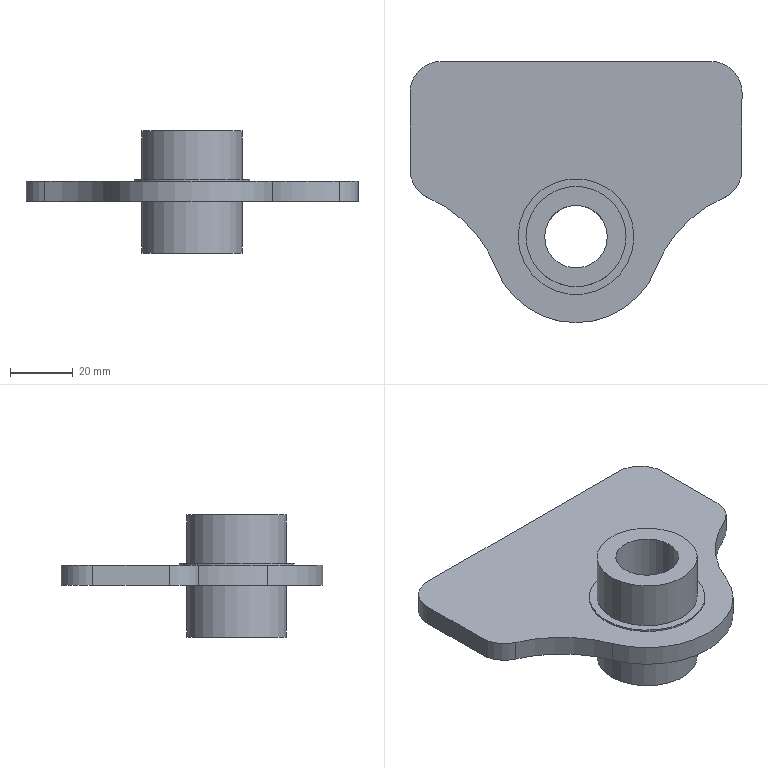NC program | NX | posted with a generic post | part box 106 x 83.448 x 39 mm
Lines 1 to 897 of 2052:
N10 G17 G21 G94 G90
(ADAPTIVE_MILLING , TOOL : D16-48-D16-100-3T-FINISH)
N12 T01 M6
N14 G53
N16 G17 G0 G90 X-29.129 Y-11.877 S3000 M3
N18 G43 Z30. H1
N20 Z3.15
N22 G94 G1 X-28.979 Y-11.865 Z2.213 F2000.
N24 X-28.829 Y-11.854 Z1.842
N26 X-28.68 Y-11.842 Z1.57
N28 X-28.53 Y-11.831 Z1.35
N30 X-28.381 Y-11.819 Z1.166
N32 X-28.231 Y-11.808 Z1.008
N34 X-28.082 Y-11.796 Z0.87
N36 X-27.932 Y-11.785 Z0.75
N38 X-27.783 Y-11.773 Z0.645
N40 X-27.633 Y-11.762 Z0.552
N42 X-27.483 Y-11.75 Z0.471
N44 X-27.334 Y-11.739 Z0.4
N46 X-27.184 Y-11.727 Z0.34
N48 X-27.035 Y-11.716 Z0.288
N50 X-26.885 Y-11.704 Z0.245
N52 X-26.736 Y-11.693 Z0.211
N54 X-26.586 Y-11.681 Z0.184
N56 X-26.436 Y-11.67 Z0.165
N58 X-26.287 Y-11.658 Z0.154
N60 X-26.137 Y-11.647 Z0.15
N62 X-24.02 Y-11.484
N64 G3 X-22.555 Y-9.578 R1.616
N66 G1 X-23.473 Y-5.647
N68 G2 X-22.056 Y9.568 R25.074
N70 X-20.662 Y-12.268 R-24.039
N72 X-23.288 Y-4.358 R24.506
N74 X-17.653 Y15.653 R24.1
N76 X-19.314 Y-13.525 R-23.593
N78 X-23.013 Y-3.231 R23.544
N80 X-13.785 Y18.59 R23.495
N82 X-17.92 Y-14.622 R-23.141
N84 X-22.633 Y-2.662 R22.849
N86 X-11.014 Y19.837 R22.99
N88 X-16.545 Y-15.504 R-22.686
N90 X-22.228 Y-2.182 R22.315
N92 X-8.532 Y20.527 R22.498
N94 X-15.335 Y-16.071 R-22.227
N96 X-21.826 Y-1.358 R21.88
N98 X-5.19 Y21.138 R21.988
N100 X-14.251 Y-16.427 R-21.762
N102 X-21.39 Y-0.363 R21.453
N104 X-1.126 Y21.266 R21.473
N106 X-12.994 Y-16.848 R-21.29
N108 X-20.917 Y0.217 R20.985
N110 X1.005 Y20.795 R20.982
N112 X-12.004 Y-16.984 R-20.813
N114 X-20.383 Y1.367 R20.542
N116 X4.974 Y19.719 R20.469
N118 X-11.011 Y-17.069 R-20.328
N120 X-19.791 Y2.388 R20.075
N122 X7.915 Y18.2 R19.96
N124 X-10.001 Y-17.112 R-19.835
N126 X-19.13 Y3.418 R19.594
N128 X10.367 Y16.335 R19.447
N130 X-9.145 Y-17.018 R19.333
N132 X-18.337 Y4.66 R19.106
N134 X12.992 Y13.643 R18.923
N136 X-8.398 Y-16.83 R18.82
N138 X-16.984 Y7.044 R18.615
N140 X17.291 Y6.061 R18.375
N142 X-8.2 Y-16.341 R18.285
N144 X-13.274 Y11.907 R18.121
N146 X-17.828 Y-0.094 R-17.828
N148 G1 X-17.825 Y0.056 Z0.154
N150 X-17.823 Y0.206 Z0.165
N152 X-17.821 Y0.356 Z0.184
N154 X-17.818 Y0.506 Z0.211
N156 X-17.816 Y0.656 Z0.245
N158 X-17.813 Y0.806 Z0.288
N160 X-17.811 Y0.956 Z0.34
N162 X-17.809 Y1.106 Z0.4
N164 X-17.806 Y1.256 Z0.471
N166 X-17.804 Y1.406 Z0.552
N168 X-17.802 Y1.556 Z0.645
N170 X-17.799 Y1.706 Z0.75
N172 X-17.797 Y1.856 Z0.87
N174 X-17.795 Y2.006 Z1.008
N176 X-17.792 Y2.156 Z1.166
N178 X-17.79 Y2.306 Z1.35
N180 X-17.788 Y2.456 Z1.57
N182 X-17.785 Y2.606 Z1.842
N184 X-17.783 Y2.756 Z2.213
N186 X-17.78 Y2.906 Z3.15
N188 G0 Z30.
(PLANAR_MILL_1_COPY , TOOL : D16-48-D16-100-3T-FINISH)
N190 X-13.655 Y22.716
N192 Z-11.9
N194 G1 X-12.158 Y23.58 Z-11.909 F1000.
N196 X-8.916 Y24.987 Z-11.928
N198 X-5.517 Y25.95 Z-11.946
N200 X-2.019 Y26.453 Z-11.965
N202 X1.514 Y26.487 Z-11.983
N204 X5.02 Y26.051 Z-12.002
N206 X8.438 Y25.152 Z-12.02
N208 X11.706 Y23.808 Z-12.039
N210 X14.766 Y22.041 Z-12.057
N212 X17.564 Y19.884 Z-12.076
N214 X20.05 Y17.373 Z-12.094
N216 X22.181 Y14.555 Z-12.113
N218 X23.919 Y11.478 Z-12.131
N220 X25.232 Y8.197 Z-12.15
N222 X26.097 Y4.772 Z-12.168
N224 X26.5 Y1.261 Z-12.187
N226 Y-1.261 Z-12.2
N228 X26.093 Y-4.794 Z-12.218
N230 X25.218 Y-8.241 Z-12.237
N232 X23.889 Y-11.54 Z-12.256
N234 X22.131 Y-14.631 Z-12.274
N236 X19.975 Y-17.46 Z-12.293
N238 X17.46 Y-19.975 Z-12.312
N240 X14.632 Y-22.13 Z-12.33
N242 X11.54 Y-23.889 Z-12.349
N244 X8.242 Y-25.217 Z-12.367
N246 X4.795 Y-26.093 Z-12.386
N248 X1.262 Y-26.5 Z-12.405
N250 X-1.261 Z-12.418
N252 X-4.087 Y-26.213 Z-12.433
N254 X-6.866 Y-25.626 Z-12.448
N256 X-9.567 Y-24.745 Z-12.462
N258 X-12.158 Y-23.58 Z-12.477
N260 X-14.342 Y-22.319 Z-12.491
N262 X-17.181 Y-20.215 Z-12.509
N264 X-19.715 Y-17.753 Z-12.528
N266 X-21.899 Y-14.975 Z-12.546
N268 X-23.695 Y-11.932 Z-12.565
N270 X-25.071 Y-8.677 Z-12.583
N272 X-26.002 Y-5.269 Z-12.602
N274 X-26.471 Y-1.767 Z-12.62
N276 Y1.767 Z-12.639
N278 X-26.002 Y5.269 Z-12.657
N280 X-25.071 Y8.677 Z-12.676
N282 X-23.695 Y11.932 Z-12.694
N284 X-21.899 Y14.975 Z-12.713
N286 X-19.715 Y17.753 Z-12.731
N288 X-17.181 Y20.215 Z-12.75
N290 X-14.342 Y22.319 Z-12.768
N292 X-12.158 Y23.58 Z-12.781
N294 X-8.916 Y24.987 Z-12.8
N296 X-5.517 Y25.95 Z-12.818
N298 X-2.019 Y26.453 Z-12.837
N300 X1.514 Y26.487 Z-12.855
N302 X5.02 Y26.051 Z-12.874
N304 X8.438 Y25.152 Z-12.892
N306 X11.706 Y23.808 Z-12.911
N308 X14.766 Y22.041 Z-12.929
N310 X17.564 Y19.884 Z-12.948
N312 X20.05 Y17.373 Z-12.966
N314 X22.181 Y14.555 Z-12.985
N316 X23.919 Y11.478 Z-13.003
N318 X25.232 Y8.197 Z-13.022
N320 X26.097 Y4.772 Z-13.04
N322 X26.5 Y1.261 Z-13.059
N324 Y-1.261 Z-13.072
N326 X26.093 Y-4.794 Z-13.091
N328 X25.218 Y-8.241 Z-13.109
N330 X23.889 Y-11.54 Z-13.128
N332 X22.131 Y-14.631 Z-13.146
N334 X19.975 Y-17.46 Z-13.165
N336 X17.46 Y-19.975 Z-13.184
N338 X14.632 Y-22.13 Z-13.202
N340 X11.54 Y-23.889 Z-13.221
N342 X8.242 Y-25.217 Z-13.24
N344 X4.795 Y-26.093 Z-13.258
N346 X1.262 Y-26.5 Z-13.277
N348 X-1.261 Z-13.29
N350 X-4.087 Y-26.213 Z-13.305
N352 X-6.866 Y-25.626 Z-13.32
N354 X-9.567 Y-24.745 Z-13.335
N356 X-12.158 Y-23.58 Z-13.35
N358 X-14.342 Y-22.319 Z-13.363
N360 X-17.181 Y-20.215 Z-13.381
N362 X-19.715 Y-17.753 Z-13.4
N364 X-21.899 Y-14.975 Z-13.418
N366 X-23.695 Y-11.932 Z-13.437
N368 X-25.071 Y-8.677 Z-13.455
N370 X-26.002 Y-5.269 Z-13.474
N372 X-26.471 Y-1.767 Z-13.492
N374 Y1.767 Z-13.511
N376 X-26.002 Y5.269 Z-13.529
N378 X-25.071 Y8.677 Z-13.548
N380 X-23.695 Y11.932 Z-13.566
N382 X-21.899 Y14.975 Z-13.585
N384 X-19.715 Y17.753 Z-13.603
N386 X-17.181 Y20.215 Z-13.622
N388 X-14.342 Y22.319 Z-13.64
N390 X-12.158 Y23.58 Z-13.653
N392 X-8.916 Y24.987 Z-13.672
N394 X-5.517 Y25.95 Z-13.69
N396 X-2.019 Y26.453 Z-13.709
N398 X1.514 Y26.487 Z-13.727
N400 X5.02 Y26.051 Z-13.746
N402 X8.438 Y25.152 Z-13.764
N404 X11.706 Y23.808 Z-13.783
N406 X14.766 Y22.041 Z-13.801
N408 X17.564 Y19.884 Z-13.82
N410 X20.05 Y17.373 Z-13.838
N412 X22.181 Y14.555 Z-13.857
N414 X23.919 Y11.478 Z-13.875
N416 X25.232 Y8.197 Z-13.894
N418 X26.097 Y4.772 Z-13.912
N420 X26.5 Y1.261 Z-13.931
N422 Y-1.261 Z-13.944
N424 X26.093 Y-4.794 Z-13.963
N426 X25.218 Y-8.241 Z-13.981
N428 X23.889 Y-11.54 Z-14.
N430 X22.131 Y-14.631 Z-14.019
N432 X19.975 Y-17.46 Z-14.037
N434 X17.46 Y-19.975 Z-14.056
N436 X14.632 Y-22.13 Z-14.075
N438 X11.54 Y-23.889 Z-14.093
N440 X8.242 Y-25.217 Z-14.112
N442 X4.795 Y-26.093 Z-14.13
N444 X1.262 Y-26.5 Z-14.149
N446 X-1.261 Z-14.162
N448 X-4.087 Y-26.213 Z-14.177
N450 X-6.866 Y-25.626 Z-14.192
N452 X-9.567 Y-24.745 Z-14.207
N454 X-12.158 Y-23.58 Z-14.222
N456 X-14.342 Y-22.319 Z-14.235
N458 X-17.181 Y-20.215 Z-14.253
N460 X-19.715 Y-17.753 Z-14.272
N462 X-21.899 Y-14.975 Z-14.29
N464 X-23.695 Y-11.932 Z-14.309
N466 X-25.071 Y-8.677 Z-14.327
N468 X-26.002 Y-5.269 Z-14.346
N470 X-26.471 Y-1.767 Z-14.364
N472 Y1.767 Z-14.383
N474 X-26.002 Y5.269 Z-14.401
N476 X-25.071 Y8.677 Z-14.42
N478 X-23.695 Y11.932 Z-14.438
N480 X-21.899 Y14.975 Z-14.457
N482 X-19.715 Y17.753 Z-14.475
N484 X-17.181 Y20.215 Z-14.494
N486 X-14.342 Y22.319 Z-14.512
N488 X-12.158 Y23.58 Z-14.526
N490 X-8.916 Y24.987 Z-14.544
N492 X-5.517 Y25.95 Z-14.563
N494 X-2.019 Y26.453 Z-14.581
N496 X1.514 Y26.487 Z-14.6
N498 X5.02 Y26.051 Z-14.618
N500 X8.438 Y25.152 Z-14.637
N502 X11.706 Y23.808 Z-14.655
N504 X14.766 Y22.041 Z-14.674
N506 X17.564 Y19.884 Z-14.692
N508 X20.05 Y17.373 Z-14.711
N510 X22.181 Y14.555 Z-14.729
N512 X23.919 Y11.478 Z-14.748
N514 X25.232 Y8.197 Z-14.766
N516 X26.097 Y4.772 Z-14.785
N518 X26.5 Y1.261 Z-14.803
N520 Y-1.261 Z-14.816
N522 X26.093 Y-4.794 Z-14.835
N524 X25.218 Y-8.241 Z-14.854
N526 X23.889 Y-11.54 Z-14.872
N528 X22.131 Y-14.631 Z-14.891
N530 X19.975 Y-17.46 Z-14.909
N532 X17.46 Y-19.975 Z-14.928
N534 X14.632 Y-22.13 Z-14.947
N536 X11.54 Y-23.889 Z-14.965
N538 X8.242 Y-25.217 Z-14.984
N540 X4.795 Y-26.093 Z-15.003
N542 X1.262 Y-26.5 Z-15.021
N544 X-1.261 Z-15.034
N546 X-4.087 Y-26.213 Z-15.049
N548 X-6.866 Y-25.626 Z-15.064
N550 X-9.567 Y-24.745 Z-15.079
N552 X-12.158 Y-23.58 Z-15.094
N554 X-14.342 Y-22.319 Z-15.107
N556 X-17.181 Y-20.215 Z-15.126
N558 X-19.715 Y-17.753 Z-15.144
N560 X-21.899 Y-14.975 Z-15.163
N562 X-23.695 Y-11.932 Z-15.181
N564 X-25.071 Y-8.677 Z-15.2
N566 X-26.002 Y-5.269 Z-15.218
N568 X-26.471 Y-1.767 Z-15.237
N570 Y1.767 Z-15.255
N572 X-26.002 Y5.269 Z-15.274
N574 X-25.071 Y8.677 Z-15.292
N576 X-23.695 Y11.932 Z-15.311
N578 X-21.899 Y14.975 Z-15.329
N580 X-19.715 Y17.753 Z-15.348
N582 X-17.181 Y20.215 Z-15.366
N584 X-14.342 Y22.319 Z-15.385
N586 X-12.158 Y23.58 Z-15.398
N588 X-8.916 Y24.987 Z-15.416
N590 X-5.517 Y25.95 Z-15.435
N592 X-2.019 Y26.453 Z-15.453
N594 X1.514 Y26.487 Z-15.472
N596 X5.02 Y26.051 Z-15.49
N598 X8.438 Y25.152 Z-15.509
N600 X11.706 Y23.808 Z-15.527
N602 X14.766 Y22.041 Z-15.546
N604 X17.564 Y19.884 Z-15.564
N606 X20.05 Y17.373 Z-15.583
N608 X22.181 Y14.555 Z-15.601
N610 X23.919 Y11.478 Z-15.62
N612 X25.232 Y8.197 Z-15.638
N614 X26.097 Y4.772 Z-15.657
N616 X26.5 Y1.261 Z-15.675
N618 Y-1.261 Z-15.689
N620 X26.093 Y-4.794 Z-15.707
N622 X25.218 Y-8.241 Z-15.726
N624 X23.889 Y-11.54 Z-15.744
N626 X22.131 Y-14.631 Z-15.763
N628 X19.975 Y-17.46 Z-15.782
N630 X17.46 Y-19.975 Z-15.8
N632 X14.632 Y-22.13 Z-15.819
N634 X11.54 Y-23.889 Z-15.838
N636 X8.242 Y-25.217 Z-15.856
N638 X4.795 Y-26.093 Z-15.875
N640 X1.262 Y-26.5 Z-15.893
N642 X0. Z-15.9
N644 G2 X-26.5 Y0. R26.5
N646 X0. Y-26.5 R-26.5
N648 G1 Z-11.9
N650 G0 Z30.
(PLANAR_MILL , TOOL : D16-48-D16-100-3T-FINISH)
N652 X-25.515 Y-5.
N654 Z3.
N656 G1 Z0.
N658 X-21.
N660 G3 X-16. Y0. R5.
N662 G2 X0. Y16. R16.
N664 X-16. Y0. R-16.
N666 G3 X-21. Y5. R5.
N668 G1 X-25.515
N670 Z3.
N672 G0 Z30.
(FLOOR_WALL , TOOL : D16-48-D16-100-3T-FINISH)
N674 X-4. Y67.
N676 Z-12.
N678 G1 Z-15.
N680 Y56.
N682 G3 X0. Y52. R4.
N684 G1 X43.
N686 G2 X49. Y46. R6.
N688 G1 Y21.463
N690 G2 X45.39 Y15.96 R6.
N692 G3 X26.498 Y0.294 R44.
N694 X-26.498 Y0.295 R26.5
N696 X-45.39 Y15.96 R44.
N698 G2 X-49. Y21.463 R6.
N700 G1 Y46.
N702 G2 X-43. Y52. R6.
N704 G1 X0.
N706 Y40.
N708 X37.
N710 Y25.243
N712 G3 X31.584 Y22.016 R56.
N714 X-31.584 Y22.016 R38.5
N716 X-37. Y25.243 R56.
N718 G1 Y40.
N720 X0.
N722 X1.
N724 G3 X5. Y44. R4.
N726 G1 Z-12.
N728 G0 Z30.
N730 X-4. Y67.
N732 Z-13.
N734 G1 Z-16.
N736 Y56.
N738 G3 X0. Y52. R4.
N740 G1 X43.
N742 G2 X49. Y46. R6.
N744 G1 Y21.463
N746 G2 X45.39 Y15.96 R6.
N748 G3 X26.498 Y0.294 R44.
N750 X-26.498 Y0.295 R26.5
N752 X-45.39 Y15.96 R44.
N754 G2 X-49. Y21.463 R6.
N756 G1 Y46.
N758 G2 X-43. Y52. R6.
N760 G1 X0.
N762 Y40.
N764 X37.
N766 Y25.243
N768 G3 X31.584 Y22.016 R56.
N770 X-31.584 Y22.016 R38.5
N772 X-37. Y25.243 R56.
N774 G1 Y40.
N776 X0.
N778 X1.
N780 G3 X5. Y44. R4.
N782 G1 Z-13.
N784 G0 Z30.
(PLANAR_MILL_1 , TOOL : D16-48-D16-100-3T-FINISH)
N786 X5.001 Y-36.156
N788 Z-14.
N790 G1 Z-16.
N792 Y-31.5
N794 G3 X0. Y-26.5 R5.
N796 G2 X-26.5 Y0. R26.5
N798 X0. Y-26.5 R-26.5
N800 G3 X-4.999 Y-31.5 R5.
N802 G1 Y-36.156
N804 Z-14.
N806 G0 Z30.
(PLANAR_MILL_4 , TOOL : D16-48-D16-100-3T-FINISH)
N808 X1.876 Y0.397
N810 Z2.
N812 G1 X1.58 Y1.109 Z1.973
N814 X0.965 Y1.671 Z1.944
N816 X0.17 Y1.922 Z1.915
N818 X-0.656 Y1.815 Z1.886
N820 X-1.244 Y1.476 Z1.862
N822 X-1.671 Y0.965 Z1.839
N824 X-1.9 Y0.339 Z1.816
N826 Y-0.339 Z1.792
N828 X-1.671 Y-0.965 Z1.769
N830 X-1.244 Y-1.476 Z1.745
N832 X-0.656 Y-1.815 Z1.722
N834 X0.17 Y-1.922 Z1.693
N836 X0.965 Y-1.671 Z1.663
N838 X1.58 Y-1.109 Z1.634
N840 X1.9 Y-0.339 Z1.605
N842 Y0.339 Z1.582
N844 X1.58 Y1.109 Z1.552
N846 X0.965 Y1.671 Z1.523
N848 X0.17 Y1.922 Z1.494
N850 X-0.656 Y1.815 Z1.465
N852 X-1.244 Y1.476 Z1.441
N854 X-1.671 Y0.965 Z1.418
N856 X-1.9 Y0.339 Z1.395
N858 Y-0.339 Z1.371
N860 X-1.671 Y-0.965 Z1.348
N862 X-1.244 Y-1.476 Z1.325
N864 X-0.656 Y-1.815 Z1.301
N866 X0.17 Y-1.922 Z1.272
N868 X0.965 Y-1.671 Z1.243
N870 X1.58 Y-1.109 Z1.214
N872 X1.9 Y-0.339 Z1.185
N874 Y0.339 Z1.161
N876 X1.58 Y1.109 Z1.132
N878 X0.965 Y1.671 Z1.103
N880 X0.17 Y1.922 Z1.074
N882 X-0.656 Y1.815 Z1.044
N884 X-1.244 Y1.476 Z1.021
N886 X-1.671 Y0.965 Z0.998
N888 X-1.9 Y0.339 Z0.974
N890 Y-0.339 Z0.951
N892 X-1.671 Y-0.965 Z0.927
N894 X-1.244 Y-1.476 Z0.904
N896 X-0.656 Y-1.815 Z0.88
N898 X0.17 Y-1.922 Z0.851
N900 X0.965 Y-1.671 Z0.822
N902 X1.58 Y-1.109 Z0.793
N904 X1.9 Y-0.339 Z0.764
N906 Y0.339 Z0.74
N908 X1.58 Y1.109 Z0.711
N910 X0.965 Y1.671 Z0.682
N912 X0.17 Y1.922 Z0.653
N914 X-0.656 Y1.815 Z0.624
N916 X-1.244 Y1.476 Z0.6
N918 X-1.671 Y0.965 Z0.577
N920 X-1.9 Y0.339 Z0.554
N922 Y-0.339 Z0.53
N924 X-1.671 Y-0.965 Z0.507
N926 X-1.244 Y-1.476 Z0.483
N928 X-0.656 Y-1.815 Z0.46
N930 X0.17 Y-1.922 Z0.431
N932 X0.965 Y-1.671 Z0.401
N934 X1.58 Y-1.109 Z0.372
N936 X1.9 Y-0.339 Z0.343
N938 Y0.339 Z0.32
N940 X1.58 Y1.109 Z0.29
N942 X0.965 Y1.671 Z0.261
N944 X0.17 Y1.922 Z0.232
N946 X-0.656 Y1.815 Z0.203
N948 X-1.244 Y1.476 Z0.179
N950 X-1.671 Y0.965 Z0.156
N952 X-1.9 Y0.339 Z0.133
N954 Y-0.339 Z0.109
N956 X-1.671 Y-0.965 Z0.086
N958 X-1.244 Y-1.476 Z0.063
N960 X-0.656 Y-1.815 Z0.039
N962 X0.17 Y-1.922 Z0.01
N964 X0.965 Y-1.671 Z-0.019
N966 X1.58 Y-1.109 Z-0.048
N968 X1.9 Y-0.339 Z-0.077
N970 Y0.339 Z-0.101
N972 X1.58 Y1.109 Z-0.13
N974 X0.965 Y1.671 Z-0.159
N976 X0.17 Y1.922 Z-0.188
N978 X-0.656 Y1.815 Z-0.218
N980 X-1.244 Y1.476 Z-0.241
N982 X-1.671 Y0.965 Z-0.264
N984 X-1.9 Y0.339 Z-0.288
N986 Y-0.339 Z-0.311
N988 X-1.671 Y-0.965 Z-0.335
N990 X-1.244 Y-1.476 Z-0.358
N992 X-0.656 Y-1.815 Z-0.382
N994 X0.17 Y-1.922 Z-0.411
N996 X0.965 Y-1.671 Z-0.44
N998 X1.58 Y-1.109 Z-0.469
N1000 X1.9 Y-0.339 Z-0.498
N1002 Y0.339 Z-0.522
N1004 X1.58 Y1.109 Z-0.551
N1006 X0.965 Y1.671 Z-0.58
N1008 X0.17 Y1.922 Z-0.609
N1010 X-0.656 Y1.815 Z-0.638
N1012 X-1.244 Y1.476 Z-0.662
N1014 X-1.671 Y0.965 Z-0.685
N1016 X-1.9 Y0.339 Z-0.708
N1018 Y-0.339 Z-0.732
N1020 X-1.671 Y-0.965 Z-0.755
N1022 X-1.244 Y-1.476 Z-0.779
N1024 X-0.656 Y-1.815 Z-0.802
N1026 X0.17 Y-1.922 Z-0.831
N1028 X0.965 Y-1.671 Z-0.861
N1030 X1.58 Y-1.109 Z-0.89
N1032 X1.9 Y-0.339 Z-0.919
N1034 Y0.339 Z-0.942
N1036 X1.58 Y1.109 Z-0.972
N1038 X0.965 Y1.671 Z-1.001
N1040 X0.17 Y1.922 Z-1.03
N1042 X-0.656 Y1.815 Z-1.059
N1044 X-1.244 Y1.476 Z-1.083
N1046 X-1.671 Y0.965 Z-1.106
N1048 X-1.9 Y0.339 Z-1.129
N1050 Y-0.339 Z-1.153
N1052 X-1.671 Y-0.965 Z-1.176
N1054 X-1.244 Y-1.476 Z-1.199
N1056 X-0.656 Y-1.815 Z-1.223
N1058 X0.17 Y-1.922 Z-1.252
N1060 X0.965 Y-1.671 Z-1.281
N1062 X1.58 Y-1.109 Z-1.31
N1064 X1.9 Y-0.339 Z-1.339
N1066 Y0.339 Z-1.363
N1068 X1.58 Y1.109 Z-1.392
N1070 X0.965 Y1.671 Z-1.421
N1072 X0.17 Y1.922 Z-1.45
N1074 X-0.656 Y1.815 Z-1.479
N1076 X-1.244 Y1.476 Z-1.503
N1078 X-1.671 Y0.965 Z-1.526
N1080 X-1.9 Y0.339 Z-1.55
N1082 Y-0.339 Z-1.573
N1084 X-1.671 Y-0.965 Z-1.597
N1086 X-1.244 Y-1.476 Z-1.62
N1088 X-0.656 Y-1.815 Z-1.644
N1090 X0.17 Y-1.922 Z-1.673
N1092 X0.965 Y-1.671 Z-1.702
N1094 X1.58 Y-1.109 Z-1.731
N1096 X1.9 Y-0.339 Z-1.76
N1098 Y0.339 Z-1.784
N1100 X1.58 Y1.109 Z-1.813
N1102 X0.965 Y1.671 Z-1.842
N1104 X0.17 Y1.922 Z-1.871
N1106 X-0.656 Y1.815 Z-1.9
N1108 X-1.244 Y1.476 Z-1.924
N1110 X-1.671 Y0.965 Z-1.947
N1112 X-1.9 Y0.339 Z-1.97
N1114 Y-0.339 Z-1.994
N1116 X-1.671 Y-0.965 Z-2.017
N1118 X-1.244 Y-1.476 Z-2.041
N1120 X-0.656 Y-1.815 Z-2.064
N1122 X0.17 Y-1.922 Z-2.093
N1124 X0.965 Y-1.671 Z-2.122
N1126 X1.58 Y-1.109 Z-2.152
N1128 X1.9 Y-0.339 Z-2.181
N1130 Y0.339 Z-2.204
N1132 X1.58 Y1.109 Z-2.233
N1134 X0.965 Y1.671 Z-2.263
N1136 X0.17 Y1.922 Z-2.292
N1138 X-0.656 Y1.815 Z-2.321
N1140 X-1.244 Y1.476 Z-2.344
N1142 X-1.671 Y0.965 Z-2.368
N1144 X-1.9 Y0.339 Z-2.391
N1146 Y-0.339 Z-2.415
N1148 X-1.671 Y-0.965 Z-2.438
N1150 X-1.244 Y-1.476 Z-2.461
N1152 X-0.656 Y-1.815 Z-2.485
N1154 X0.17 Y-1.922 Z-2.514
N1156 X0.965 Y-1.671 Z-2.543
N1158 X1.58 Y-1.109 Z-2.572
N1160 X1.9 Y-0.339 Z-2.601
N1162 Y0.339 Z-2.625
N1164 X1.58 Y1.109 Z-2.654
N1166 X0.965 Y1.671 Z-2.683
N1168 X0.17 Y1.922 Z-2.712
N1170 X-0.656 Y1.815 Z-2.741
N1172 X-1.244 Y1.476 Z-2.765
N1174 X-1.671 Y0.965 Z-2.788
N1176 X-1.9 Y0.339 Z-2.812
N1178 Y-0.339 Z-2.835
N1180 X-1.671 Y-0.965 Z-2.859
N1182 X-1.244 Y-1.476 Z-2.882
N1184 X-0.656 Y-1.815 Z-2.906
N1186 X0.17 Y-1.922 Z-2.935
N1188 X0.965 Y-1.671 Z-2.964
N1190 X1.58 Y-1.109 Z-2.993
N1192 X1.9 Y-0.339 Z-3.022
N1194 Y0.339 Z-3.046
N1196 X1.58 Y1.109 Z-3.075
N1198 X0.965 Y1.671 Z-3.104
N1200 X0.17 Y1.922 Z-3.133
N1202 X-0.656 Y1.815 Z-3.162
N1204 X-1.244 Y1.476 Z-3.186
N1206 X-1.671 Y0.965 Z-3.209
N1208 X-1.9 Y0.339 Z-3.232
N1210 Y-0.339 Z-3.256
N1212 X-1.671 Y-0.965 Z-3.279
N1214 X-1.244 Y-1.476 Z-3.303
N1216 X-0.656 Y-1.815 Z-3.326
N1218 X0.17 Y-1.922 Z-3.355
N1220 X0.965 Y-1.671 Z-3.384
N1222 X1.58 Y-1.109 Z-3.414
N1224 X1.9 Y-0.339 Z-3.443
N1226 Y0.339 Z-3.466
N1228 X1.58 Y1.109 Z-3.495
N1230 X0.965 Y1.671 Z-3.525
N1232 X0.17 Y1.922 Z-3.554
N1234 X-0.656 Y1.815 Z-3.583
N1236 X-1.244 Y1.476 Z-3.606
N1238 X-1.671 Y0.965 Z-3.63
N1240 X-1.9 Y0.339 Z-3.653
N1242 Y-0.339 Z-3.677
N1244 X-1.671 Y-0.965 Z-3.7
N1246 X-1.244 Y-1.476 Z-3.723
N1248 X-0.656 Y-1.815 Z-3.747
N1250 X0.17 Y-1.922 Z-3.776
N1252 X0.965 Y-1.671 Z-3.805
N1254 X1.58 Y-1.109 Z-3.834
N1256 X1.9 Y-0.339 Z-3.863
N1258 Y0.339 Z-3.887
N1260 X1.58 Y1.109 Z-3.916
N1262 X0.965 Y1.671 Z-3.945
N1264 X0.17 Y1.922 Z-3.974
N1266 X-0.656 Y1.815 Z-4.003
N1268 X-1.244 Y1.476 Z-4.027
N1270 X-1.671 Y0.965 Z-4.05
N1272 X-1.9 Y0.339 Z-4.074
N1274 Y-0.339 Z-4.097
N1276 X-1.671 Y-0.965 Z-4.121
N1278 X-1.244 Y-1.476 Z-4.144
N1280 X-0.656 Y-1.815 Z-4.168
N1282 X0.17 Y-1.922 Z-4.197
N1284 X0.965 Y-1.671 Z-4.226
N1286 X1.58 Y-1.109 Z-4.255
N1288 X1.9 Y-0.339 Z-4.284
N1290 Y0.339 Z-4.308
N1292 X1.58 Y1.109 Z-4.337
N1294 X0.965 Y1.671 Z-4.366
N1296 X0.17 Y1.922 Z-4.395
N1298 X-0.656 Y1.815 Z-4.424
N1300 X-1.244 Y1.476 Z-4.448
N1302 X-1.671 Y0.965 Z-4.471
N1304 X-1.9 Y0.339 Z-4.494
N1306 Y-0.339 Z-4.518
N1308 X-1.671 Y-0.965 Z-4.541
N1310 X-1.244 Y-1.476 Z-4.565
N1312 X-0.656 Y-1.815 Z-4.588
N1314 X0.17 Y-1.922 Z-4.617
N1316 X0.965 Y-1.671 Z-4.646
N1318 X1.58 Y-1.109 Z-4.676
N1320 X1.9 Y-0.339 Z-4.705
N1322 Y0.339 Z-4.728
N1324 X1.58 Y1.109 Z-4.757
N1326 X0.965 Y1.671 Z-4.787
N1328 X0.17 Y1.922 Z-4.816
N1330 X-0.656 Y1.815 Z-4.845
N1332 X-1.244 Y1.476 Z-4.868
N1334 X-1.671 Y0.965 Z-4.892
N1336 X-1.9 Y0.339 Z-4.915
N1338 Y-0.339 Z-4.939
N1340 X-1.671 Y-0.965 Z-4.962
N1342 X-1.244 Y-1.476 Z-4.985
N1344 X-0.656 Y-1.815 Z-5.009
N1346 X0.17 Y-1.922 Z-5.038
N1348 X0.965 Y-1.671 Z-5.067
N1350 X1.58 Y-1.109 Z-5.096
N1352 X1.9 Y-0.339 Z-5.125
N1354 Y0.339 Z-5.149
N1356 X1.58 Y1.109 Z-5.178
N1358 X0.965 Y1.671 Z-5.207
N1360 X0.17 Y1.922 Z-5.236
N1362 X-0.656 Y1.815 Z-5.265
N1364 X-1.244 Y1.476 Z-5.289
N1366 X-1.671 Y0.965 Z-5.312
N1368 X-1.9 Y0.339 Z-5.336
N1370 Y-0.339 Z-5.359
N1372 X-1.671 Y-0.965 Z-5.383
N1374 X-1.244 Y-1.476 Z-5.406
N1376 X-0.656 Y-1.815 Z-5.43
N1378 X0.17 Y-1.922 Z-5.459
N1380 X0.965 Y-1.671 Z-5.488
N1382 X1.58 Y-1.109 Z-5.517
N1384 X1.9 Y-0.339 Z-5.546
N1386 Y0.339 Z-5.57
N1388 X1.58 Y1.109 Z-5.599
N1390 X0.965 Y1.671 Z-5.628
N1392 X0.17 Y1.922 Z-5.657
N1394 X-0.656 Y1.815 Z-5.686
N1396 X-1.244 Y1.476 Z-5.71
N1398 X-1.671 Y0.965 Z-5.733
N1400 X-1.9 Y0.339 Z-5.756
N1402 Y-0.339 Z-5.78
N1404 X-1.671 Y-0.965 Z-5.803
N1406 X-1.244 Y-1.476 Z-5.826
N1408 X-0.656 Y-1.815 Z-5.85
N1410 X0.17 Y-1.922 Z-5.879
N1412 X0.965 Y-1.671 Z-5.908
N1414 X1.58 Y-1.109 Z-5.937
N1416 X1.9 Y-0.339 Z-5.967
N1418 Y0.339 Z-5.99
N1420 X1.58 Y1.109 Z-6.019
N1422 X0.965 Y1.671 Z-6.048
N1424 X0.17 Y1.922 Z-6.078
N1426 X-0.656 Y1.815 Z-6.107
N1428 X-1.244 Y1.476 Z-6.13
N1430 X-1.671 Y0.965 Z-6.154
N1432 X-1.9 Y0.339 Z-6.177
N1434 Y-0.339 Z-6.201
N1436 X-1.671 Y-0.965 Z-6.224
N1438 X-1.244 Y-1.476 Z-6.247
N1440 X-0.656 Y-1.815 Z-6.271
N1442 X0.17 Y-1.922 Z-6.3
N1444 X0.965 Y-1.671 Z-6.329
N1446 X1.58 Y-1.109 Z-6.358
N1448 X1.9 Y-0.339 Z-6.387
N1450 Y0.339 Z-6.411
N1452 X1.58 Y1.109 Z-6.44
N1454 X0.965 Y1.671 Z-6.469
N1456 X0.17 Y1.922 Z-6.498
N1458 X-0.656 Y1.815 Z-6.527
N1460 X-1.244 Y1.476 Z-6.551
N1462 X-1.671 Y0.965 Z-6.574
N1464 X-1.9 Y0.339 Z-6.598
N1466 Y-0.339 Z-6.621
N1468 X-1.671 Y-0.965 Z-6.645
N1470 X-1.244 Y-1.476 Z-6.668
N1472 X-0.656 Y-1.815 Z-6.691
N1474 X0.17 Y-1.922 Z-6.721
N1476 X0.965 Y-1.671 Z-6.75
N1478 X1.58 Y-1.109 Z-6.779
N1480 X1.9 Y-0.339 Z-6.808
N1482 Y0.339 Z-6.832
N1484 X1.58 Y1.109 Z-6.861
N1486 X0.965 Y1.671 Z-6.89
N1488 X0.17 Y1.922 Z-6.919
N1490 X-0.656 Y1.815 Z-6.948
N1492 X-1.244 Y1.476 Z-6.972
N1494 X-1.671 Y0.965 Z-6.995
N1496 X-1.9 Y0.339 Z-7.018
N1498 Y-0.339 Z-7.042
N1500 X-1.671 Y-0.965 Z-7.065
N1502 X-1.244 Y-1.476 Z-7.088
N1504 X-0.656 Y-1.815 Z-7.112
N1506 X0.17 Y-1.922 Z-7.141
N1508 X0.965 Y-1.671 Z-7.17
N1510 X1.58 Y-1.109 Z-7.199
N1512 X1.9 Y-0.339 Z-7.229
N1514 Y0.339 Z-7.252
N1516 X1.58 Y1.109 Z-7.281
N1518 X0.965 Y1.671 Z-7.31
N1520 X0.17 Y1.922 Z-7.34
N1522 X-0.656 Y1.815 Z-7.369
N1524 X-1.244 Y1.476 Z-7.392
N1526 X-1.671 Y0.965 Z-7.416
N1528 X-1.9 Y0.339 Z-7.439
N1530 Y-0.339 Z-7.463
N1532 X-1.671 Y-0.965 Z-7.486
N1534 X-1.244 Y-1.476 Z-7.509
N1536 X-0.656 Y-1.815 Z-7.533
N1538 X0.17 Y-1.922 Z-7.562
N1540 X0.965 Y-1.671 Z-7.591
N1542 X1.58 Y-1.109 Z-7.62
N1544 X1.9 Y-0.339 Z-7.649
N1546 Y0.339 Z-7.673
N1548 X1.58 Y1.109 Z-7.702
N1550 X0.965 Y1.671 Z-7.731
N1552 X0.17 Y1.922 Z-7.76
N1554 X-0.656 Y1.815 Z-7.789
N1556 X-1.244 Y1.476 Z-7.813
N1558 X-1.671 Y0.965 Z-7.836
N1560 X-1.9 Y0.339 Z-7.86
N1562 Y-0.339 Z-7.883
N1564 X-1.671 Y-0.965 Z-7.907
N1566 X-1.244 Y-1.476 Z-7.93
N1568 X-0.656 Y-1.815 Z-7.953
N1570 X0.17 Y-1.922 Z-7.983
N1572 X0.965 Y-1.671 Z-8.012
N1574 X1.58 Y-1.109 Z-8.041
N1576 X1.9 Y-0.339 Z-8.07
N1578 Y0.339 Z-8.094
N1580 X1.58 Y1.109 Z-8.123
N1582 X0.965 Y1.671 Z-8.152
N1584 X0.17 Y1.922 Z-8.181
N1586 X-0.656 Y1.815 Z-8.21
N1588 X-1.244 Y1.476 Z-8.234
N1590 X-1.671 Y0.965 Z-8.257
N1592 X-1.9 Y0.339 Z-8.28
N1594 Y-0.339 Z-8.304
N1596 X-1.671 Y-0.965 Z-8.327
N1598 X-1.244 Y-1.476 Z-8.35
N1600 X-0.656 Y-1.815 Z-8.374
N1602 X0.17 Y-1.922 Z-8.403
N1604 X0.965 Y-1.671 Z-8.432
N1606 X1.58 Y-1.109 Z-8.461
N1608 X1.9 Y-0.339 Z-8.491
N1610 Y0.339 Z-8.514
N1612 X1.58 Y1.109 Z-8.543
N1614 X0.965 Y1.671 Z-8.572
N1616 X0.17 Y1.922 Z-8.602
N1618 X-0.656 Y1.815 Z-8.631
N1620 X-1.244 Y1.476 Z-8.654
N1622 X-1.671 Y0.965 Z-8.678
N1624 X-1.9 Y0.339 Z-8.701
N1626 Y-0.339 Z-8.725
N1628 X-1.671 Y-0.965 Z-8.748
N1630 X-1.244 Y-1.476 Z-8.771
N1632 X-0.656 Y-1.815 Z-8.795
N1634 X0.17 Y-1.922 Z-8.824
N1636 X0.965 Y-1.671 Z-8.853
N1638 X1.58 Y-1.109 Z-8.882
N1640 X1.9 Y-0.339 Z-8.911
N1642 Y0.339 Z-8.935
N1644 X1.58 Y1.109 Z-8.964
N1646 X0.965 Y1.671 Z-8.993
N1648 X0.17 Y1.922 Z-9.022
N1650 X-0.656 Y1.815 Z-9.051
N1652 X-1.244 Y1.476 Z-9.075
N1654 X-1.671 Y0.965 Z-9.098
N1656 X-1.9 Y0.339 Z-9.122
N1658 Y-0.339 Z-9.145
N1660 X-1.671 Y-0.965 Z-9.168
N1662 X-1.244 Y-1.476 Z-9.192
N1664 X-0.656 Y-1.815 Z-9.215
N1666 X0.17 Y-1.922 Z-9.245
N1668 X0.965 Y-1.671 Z-9.274
N1670 X1.58 Y-1.109 Z-9.303
N1672 X1.9 Y-0.339 Z-9.332
N1674 Y0.339 Z-9.356
N1676 X1.58 Y1.109 Z-9.385
N1678 X0.965 Y1.671 Z-9.414
N1680 X0.17 Y1.922 Z-9.443
N1682 X-0.656 Y1.815 Z-9.472
N1684 X-1.244 Y1.476 Z-9.496
N1686 X-1.671 Y0.965 Z-9.519
N1688 X-1.9 Y0.339 Z-9.542
N1690 Y-0.339 Z-9.566
N1692 X-1.671 Y-0.965 Z-9.589
N1694 X-1.244 Y-1.476 Z-9.612
N1696 X-0.656 Y-1.815 Z-9.636
N1698 X0.17 Y-1.922 Z-9.665
N1700 X0.965 Y-1.671 Z-9.694
N1702 X1.58 Y-1.109 Z-9.723
N1704 X1.9 Y-0.339 Z-9.753
N1706 Y0.339 Z-9.776
N1708 X1.58 Y1.109 Z-9.805
N1710 X0.965 Y1.671 Z-9.834
N1712 X0.17 Y1.922 Z-9.864
N1714 X-0.656 Y1.815 Z-9.893
N1716 X-1.244 Y1.476 Z-9.916
N1718 X-1.671 Y0.965 Z-9.94
N1720 X-1.9 Y0.339 Z-9.963
N1722 Y-0.339 Z-9.987
N1724 X-1.671 Y-0.965 Z-10.01
N1726 X-1.244 Y-1.476 Z-10.033
N1728 X-0.656 Y-1.815 Z-10.057
N1730 X0.17 Y-1.922 Z-10.086
N1732 X0.965 Y-1.671 Z-10.115
N1734 X1.58 Y-1.109 Z-10.144
N1736 X1.9 Y-0.339 Z-10.173
N1738 Y0.339 Z-10.197
N1740 X1.58 Y1.109 Z-10.226
N1742 X0.965 Y1.671 Z-10.255
N1744 X0.17 Y1.922 Z-10.284
N1746 X-0.656 Y1.815 Z-10.313
N1748 X-1.244 Y1.476 Z-10.337
N1750 X-1.671 Y0.965 Z-10.36
N1752 X-1.9 Y0.339 Z-10.383
N1754 Y-0.339 Z-10.407
N1756 X-1.671 Y-0.965 Z-10.43
N1758 X-1.244 Y-1.476 Z-10.454
N1760 X-0.656 Y-1.815 Z-10.477
N1762 X0.17 Y-1.922 Z-10.507